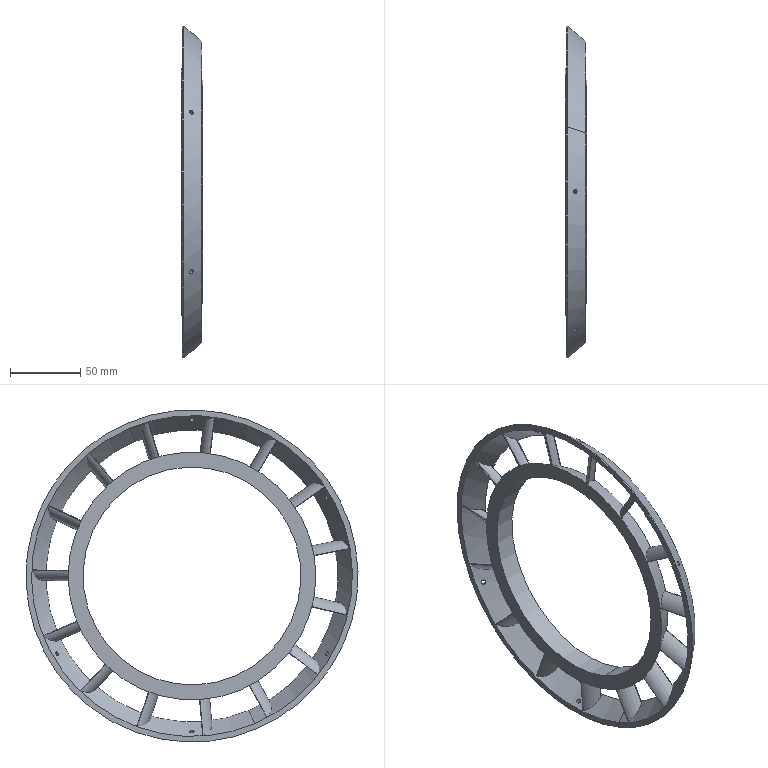Part | STEP file | Completa.sldasm-Part-59_Valor predeterminado | 1 solid | 99 faces | box 14.996 x 237.027 x 237.027 mm | volume 98651 mm3 | cylinder 89 | cone 6 | plane 4 | commonest cylinder face diameters 2 x30 0.4 x15 21.303 x15 35.24 x15 3.22 x10 155.5 x2